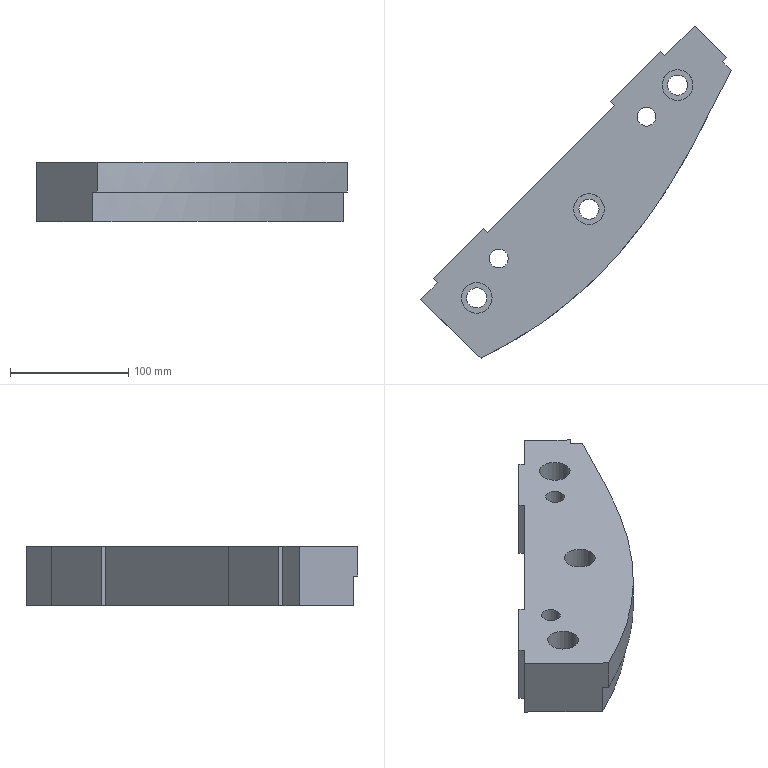Part | NX | features solid 2 | 1 solid | 32 faces | box 263.082 x 280.883 x 50 mm | volume 1203594 mm3 | plane 21 | cylinder 8 | spline 3 | commonest cylinder face diameters 17 x3 26 x3 16 x2
STEP:
#1=CARTESIAN_POINT('',(531.946,-303.622,-50.));
#2=VERTEX_POINT('',#1);
#3=CARTESIAN_POINT('',(528.349,-300.149,-50.));
#4=VERTEX_POINT('',#3);
#5=CARTESIAN_POINT('',(535.7,-307.247,-50.));
#6=DIRECTION('',(-0.7193,0.6947,0.));
#7=VECTOR('',#6,1000.);
#8=LINE('',#5,#7);
#9=EDGE_CURVE('',#2,#4,#8,.T.);
#10=ORIENTED_EDGE('',*,*,#9,.T.);
#11=CARTESIAN_POINT('',(528.349,-300.149,0.));
#12=VERTEX_POINT('',#11);
#13=CARTESIAN_POINT('',(528.349,-300.149,-50.));
#14=DIRECTION('',(0.,0.,1.));
#15=VECTOR('',#14,1000.);
#16=LINE('',#13,#15);
#17=EDGE_CURVE('',#4,#12,#16,.T.);
#18=ORIENTED_EDGE('',*,*,#17,.T.);
#19=CARTESIAN_POINT('',(535.7,-307.247,0.));
#20=VERTEX_POINT('',#19);
#21=CARTESIAN_POINT('',(535.7,-307.247,0.));
#22=DIRECTION('',(-0.7193,0.6947,0.));
#23=VECTOR('',#22,1000.);
#24=LINE('',#21,#23);
#25=EDGE_CURVE('',#20,#12,#24,.T.);
#26=ORIENTED_EDGE('',*,*,#25,.F.);
#27=CARTESIAN_POINT('',(535.7,-307.247,-25.));
#28=VERTEX_POINT('',#27);
#29=CARTESIAN_POINT('',(535.7,-307.247,-50.));
#30=DIRECTION('',(0.,0.,1.));
#31=VECTOR('',#30,1000.);
#32=LINE('',#29,#31);
#33=EDGE_CURVE('',#28,#20,#32,.T.);
#34=ORIENTED_EDGE('',*,*,#33,.F.);
#35=CARTESIAN_POINT('',(531.946,-303.622,-25.));
#36=VERTEX_POINT('',#35);
#37=CARTESIAN_POINT('',(535.7,-307.247,-25.));
#38=DIRECTION('',(0.7193,-0.6947,0.));
#39=VECTOR('',#38,1000.);
#40=LINE('',#37,#39);
#41=EDGE_CURVE('',#36,#28,#40,.T.);
#42=ORIENTED_EDGE('',*,*,#41,.F.);
#43=CARTESIAN_POINT('',(531.946,-303.622,-42.5));
#44=DIRECTION('',(0.,0.,-1.));
#45=VECTOR('',#44,1000.);
#46=LINE('',#43,#45);
#47=EDGE_CURVE('',#36,#2,#46,.T.);
#48=ORIENTED_EDGE('',*,*,#47,.T.);
#49=EDGE_LOOP('',(#10,#18,#26,#34,#42,#48));
#50=FACE_BOUND('',#49,.T.);
#51=CARTESIAN_POINT('',(535.7,-307.247,-50.));
#52=DIRECTION('',(0.6947,0.7193,0.));
#53=DIRECTION('',(-0.7193,0.6947,0.));
#54=AXIS2_PLACEMENT_3D('',#51,#52,#53);
#55=PLANE('',#54);
#56=ADVANCED_FACE('',(#50),#55,.T.);
#57=CARTESIAN_POINT('',(504.099,-269.78,-50.));
#58=VERTEX_POINT('',#57);
#59=CARTESIAN_POINT('',(479.349,-294.529,-50.));
#60=VERTEX_POINT('',#59);
#61=CARTESIAN_POINT('',(500.563,-273.316,-50.));
#62=DIRECTION('',(-0.7071,-0.7071,0.));
#63=VECTOR('',#62,1000.);
#64=LINE('',#61,#63);
#65=EDGE_CURVE('',#58,#60,#64,.T.);
#66=ORIENTED_EDGE('',*,*,#65,.T.);
#67=CARTESIAN_POINT('',(479.349,-294.529,0.));
#68=VERTEX_POINT('',#67);
#69=CARTESIAN_POINT('',(479.349,-294.529,-50.));
#70=DIRECTION('',(0.,0.,1.));
#71=VECTOR('',#70,1000.);
#72=LINE('',#69,#71);
#73=EDGE_CURVE('',#60,#68,#72,.T.);
#74=ORIENTED_EDGE('',*,*,#73,.T.);
#75=CARTESIAN_POINT('',(504.099,-269.78,0.));
#76=VERTEX_POINT('',#75);
#77=CARTESIAN_POINT('',(500.563,-273.316,0.));
#78=DIRECTION('',(-0.7071,-0.7071,0.));
#79=VECTOR('',#78,1000.);
#80=LINE('',#77,#79);
#81=EDGE_CURVE('',#76,#68,#80,.T.);
#82=ORIENTED_EDGE('',*,*,#81,.F.);
#83=CARTESIAN_POINT('',(504.099,-269.78,-50.));
#84=DIRECTION('',(0.,0.,1.));
#85=VECTOR('',#84,1000.);
#86=LINE('',#83,#85);
#87=EDGE_CURVE('',#58,#76,#86,.T.);
#88=ORIENTED_EDGE('',*,*,#87,.F.);
#89=EDGE_LOOP('',(#66,#74,#82,#88));
#90=FACE_BOUND('',#89,.T.);
#91=CARTESIAN_POINT('',(500.563,-273.316,-50.));
#92=DIRECTION('',(-0.7071,0.7071,0.));
#93=DIRECTION('',(-0.7071,-0.7071,0.));
#94=AXIS2_PLACEMENT_3D('',#91,#92,#93);
#95=PLANE('',#94);
#96=ADVANCED_FACE('',(#90),#95,.T.);
#97=CARTESIAN_POINT('',(436.923,-336.955,-50.));
#98=VERTEX_POINT('',#97);
#99=CARTESIAN_POINT('',(436.923,-336.955,0.));
#100=VERTEX_POINT('',#99);
#101=CARTESIAN_POINT('',(436.923,-336.955,-50.));
#102=DIRECTION('',(0.,0.,1.));
#103=VECTOR('',#102,1000.);
#104=LINE('',#101,#103);
#105=EDGE_CURVE('',#98,#100,#104,.T.);
#106=ORIENTED_EDGE('',*,*,#105,.F.);
#107=CARTESIAN_POINT('',(329.186,-444.692,-50.));
#108=VERTEX_POINT('',#107);
#109=CARTESIAN_POINT('',(500.563,-273.316,-50.));
#110=DIRECTION('',(-0.7071,-0.7071,0.));
#111=VECTOR('',#110,1000.);
#112=LINE('',#109,#111);
#113=EDGE_CURVE('',#98,#108,#112,.T.);
#114=ORIENTED_EDGE('',*,*,#113,.T.);
#115=CARTESIAN_POINT('',(329.186,-444.692,0.));
#116=VERTEX_POINT('',#115);
#117=CARTESIAN_POINT('',(329.186,-444.692,-50.));
#118=DIRECTION('',(0.,0.,1.));
#119=VECTOR('',#118,1000.);
#120=LINE('',#117,#119);
#121=EDGE_CURVE('',#108,#116,#120,.T.);
#122=ORIENTED_EDGE('',*,*,#121,.T.);
#123=CARTESIAN_POINT('',(500.563,-273.316,0.));
#124=DIRECTION('',(-0.7071,-0.7071,0.));
#125=VECTOR('',#124,1000.);
#126=LINE('',#123,#125);
#127=EDGE_CURVE('',#100,#116,#126,.T.);
#128=ORIENTED_EDGE('',*,*,#127,.F.);
#129=EDGE_LOOP('',(#106,#114,#122,#128));
#130=FACE_BOUND('',#129,.T.);
#131=CARTESIAN_POINT('',(500.563,-273.316,-50.));
#132=DIRECTION('',(-0.7071,0.7071,0.));
#133=DIRECTION('',(-0.7071,-0.7071,0.));
#134=AXIS2_PLACEMENT_3D('',#131,#132,#133);
#135=PLANE('',#134);
#136=ADVANCED_FACE('',(#130),#135,.T.);
#137=CARTESIAN_POINT('',(323.774,-550.663,-25.));
#138=VERTEX_POINT('',#137);
#139=CARTESIAN_POINT('',(319.947,-546.966,-25.));
#140=VERTEX_POINT('',#139);
#141=CARTESIAN_POINT('',(272.617,-501.261,-25.));
#142=DIRECTION('',(-0.7193,0.6947,0.));
#143=VECTOR('',#142,1000.);
#144=LINE('',#141,#143);
#145=EDGE_CURVE('',#138,#140,#144,.T.);
#146=ORIENTED_EDGE('',*,*,#145,.F.);
#147=CARTESIAN_POINT('',(323.774,-550.663,0.));
#148=VERTEX_POINT('',#147);
#149=CARTESIAN_POINT('',(323.774,-550.663,-50.));
#150=DIRECTION('',(0.,0.,1.));
#151=VECTOR('',#150,1000.);
#152=LINE('',#149,#151);
#153=EDGE_CURVE('',#138,#148,#152,.T.);
#154=ORIENTED_EDGE('',*,*,#153,.T.);
#155=CARTESIAN_POINT('',(272.617,-501.261,0.));
#156=VERTEX_POINT('',#155);
#157=CARTESIAN_POINT('',(272.617,-501.261,0.));
#158=DIRECTION('',(0.7193,-0.6947,0.));
#159=VECTOR('',#158,1000.);
#160=LINE('',#157,#159);
#161=EDGE_CURVE('',#156,#148,#160,.T.);
#162=ORIENTED_EDGE('',*,*,#161,.F.);
#163=CARTESIAN_POINT('',(272.617,-501.261,-50.));
#164=VERTEX_POINT('',#163);
#165=CARTESIAN_POINT('',(272.617,-501.261,-50.));
#166=DIRECTION('',(0.,0.,1.));
#167=VECTOR('',#166,1000.);
#168=LINE('',#165,#167);
#169=EDGE_CURVE('',#164,#156,#168,.T.);
#170=ORIENTED_EDGE('',*,*,#169,.F.);
#171=CARTESIAN_POINT('',(319.947,-546.966,-50.));
#172=VERTEX_POINT('',#171);
#173=CARTESIAN_POINT('',(272.617,-501.261,-50.));
#174=DIRECTION('',(0.7193,-0.6947,0.));
#175=VECTOR('',#174,1000.);
#176=LINE('',#173,#175);
#177=EDGE_CURVE('',#164,#172,#176,.T.);
#178=ORIENTED_EDGE('',*,*,#177,.T.);
#179=CARTESIAN_POINT('',(319.947,-546.966,-42.5));
#180=DIRECTION('',(0.,0.,-1.));
#181=VECTOR('',#180,1000.);
#182=LINE('',#179,#181);
#183=EDGE_CURVE('',#172,#140,#182,.F.);
#184=ORIENTED_EDGE('',*,*,#183,.T.);
#185=EDGE_LOOP('',(#146,#154,#162,#170,#178,#184));
#186=FACE_BOUND('',#185,.T.);
#187=CARTESIAN_POINT('',(272.617,-501.261,-50.));
#188=DIRECTION('',(-0.6947,-0.7193,0.));
#189=DIRECTION('',(0.7193,-0.6947,0.));
#190=AXIS2_PLACEMENT_3D('',#187,#188,#189);
#191=PLANE('',#190);
#192=ADVANCED_FACE('',(#186),#191,.T.);
#193=CARTESIAN_POINT('',(286.76,-487.119,-50.));
#194=VERTEX_POINT('',#193);
#195=CARTESIAN_POINT('',(286.76,-487.119,0.));
#196=VERTEX_POINT('',#195);
#197=CARTESIAN_POINT('',(286.76,-487.119,-50.));
#198=DIRECTION('',(0.,0.,1.));
#199=VECTOR('',#198,1000.);
#200=LINE('',#197,#199);
#201=EDGE_CURVE('',#194,#196,#200,.T.);
#202=ORIENTED_EDGE('',*,*,#201,.F.);
#203=CARTESIAN_POINT('',(500.563,-273.316,-50.));
#204=DIRECTION('',(-0.7071,-0.7071,0.));
#205=VECTOR('',#204,1000.);
#206=LINE('',#203,#205);
#207=EDGE_CURVE('',#194,#164,#206,.T.);
#208=ORIENTED_EDGE('',*,*,#207,.T.);
#209=ORIENTED_EDGE('',*,*,#169,.T.);
#210=CARTESIAN_POINT('',(500.563,-273.316,0.));
#211=DIRECTION('',(-0.7071,-0.7071,0.));
#212=VECTOR('',#211,1000.);
#213=LINE('',#210,#212);
#214=EDGE_CURVE('',#196,#156,#213,.T.);
#215=ORIENTED_EDGE('',*,*,#214,.F.);
#216=EDGE_LOOP('',(#202,#208,#209,#215));
#217=FACE_BOUND('',#216,.T.);
#218=CARTESIAN_POINT('',(500.563,-273.316,-50.));
#219=DIRECTION('',(-0.7071,0.7071,0.));
#220=DIRECTION('',(-0.7071,-0.7071,0.));
#221=AXIS2_PLACEMENT_3D('',#218,#219,#220);
#222=PLANE('',#221);
#223=ADVANCED_FACE('',(#217),#222,.T.);
#224=CARTESIAN_POINT('',(325.65,-441.157,-50.));
#225=VERTEX_POINT('',#224);
#226=CARTESIAN_POINT('',(325.65,-441.157,0.));
#227=VERTEX_POINT('',#226);
#228=CARTESIAN_POINT('',(325.65,-441.157,-50.));
#229=DIRECTION('',(0.,0.,1.));
#230=VECTOR('',#229,1000.);
#231=LINE('',#228,#230);
#232=EDGE_CURVE('',#225,#227,#231,.T.);
#233=ORIENTED_EDGE('',*,*,#232,.T.);
#234=CARTESIAN_POINT('',(329.186,-444.692,0.));
#235=DIRECTION('',(-0.7071,0.7071,0.));
#236=VECTOR('',#235,1000.);
#237=LINE('',#234,#236);
#238=EDGE_CURVE('',#116,#227,#237,.T.);
#239=ORIENTED_EDGE('',*,*,#238,.F.);
#240=ORIENTED_EDGE('',*,*,#121,.F.);
#241=CARTESIAN_POINT('',(329.186,-444.692,-50.));
#242=DIRECTION('',(-0.7071,0.7071,0.));
#243=VECTOR('',#242,1000.);
#244=LINE('',#241,#243);
#245=EDGE_CURVE('',#108,#225,#244,.T.);
#246=ORIENTED_EDGE('',*,*,#245,.T.);
#247=EDGE_LOOP('',(#233,#239,#240,#246));
#248=FACE_BOUND('',#247,.T.);
#249=CARTESIAN_POINT('',(329.186,-444.692,-50.));
#250=DIRECTION('',(-0.7071,-0.7071,0.));
#251=DIRECTION('',(0.7071,-0.7071,0.));
#252=AXIS2_PLACEMENT_3D('',#249,#250,#251);
#253=PLANE('',#252);
#254=ADVANCED_FACE('',(#248),#253,.F.);
#255=CARTESIAN_POINT('',(283.224,-483.583,-50.));
#256=VERTEX_POINT('',#255);
#257=CARTESIAN_POINT('',(283.224,-483.583,0.));
#258=VERTEX_POINT('',#257);
#259=CARTESIAN_POINT('',(283.224,-483.583,-50.));
#260=DIRECTION('',(0.,0.,1.));
#261=VECTOR('',#260,1000.);
#262=LINE('',#259,#261);
#263=EDGE_CURVE('',#256,#258,#262,.T.);
#264=ORIENTED_EDGE('',*,*,#263,.F.);
#265=CARTESIAN_POINT('',(286.76,-487.119,-50.));
#266=DIRECTION('',(-0.7071,0.7071,0.));
#267=VECTOR('',#266,1000.);
#268=LINE('',#265,#267);
#269=EDGE_CURVE('',#194,#256,#268,.T.);
#270=ORIENTED_EDGE('',*,*,#269,.F.);
#271=ORIENTED_EDGE('',*,*,#201,.T.);
#272=CARTESIAN_POINT('',(286.76,-487.119,0.));
#273=DIRECTION('',(-0.7071,0.7071,0.));
#274=VECTOR('',#273,1000.);
#275=LINE('',#272,#274);
#276=EDGE_CURVE('',#196,#258,#275,.T.);
#277=ORIENTED_EDGE('',*,*,#276,.T.);
#278=EDGE_LOOP('',(#264,#270,#271,#277));
#279=FACE_BOUND('',#278,.T.);
#280=CARTESIAN_POINT('',(286.76,-487.119,-50.));
#281=DIRECTION('',(-0.7071,-0.7071,0.));
#282=DIRECTION('',(0.7071,-0.7071,0.));
#283=AXIS2_PLACEMENT_3D('',#280,#281,#282);
#284=PLANE('',#283);
#285=ADVANCED_FACE('',(#279),#284,.T.);
#286=CARTESIAN_POINT('',(325.65,-441.157,0.));
#287=DIRECTION('',(-0.7071,-0.7071,0.));
#288=VECTOR('',#287,1000.);
#289=LINE('',#286,#288);
#290=EDGE_CURVE('',#227,#258,#289,.T.);
#291=ORIENTED_EDGE('',*,*,#290,.F.);
#292=ORIENTED_EDGE('',*,*,#232,.F.);
#293=CARTESIAN_POINT('',(325.65,-441.157,-50.));
#294=DIRECTION('',(-0.7071,-0.7071,0.));
#295=VECTOR('',#294,1000.);
#296=LINE('',#293,#295);
#297=EDGE_CURVE('',#225,#256,#296,.T.);
#298=ORIENTED_EDGE('',*,*,#297,.T.);
#299=ORIENTED_EDGE('',*,*,#263,.T.);
#300=EDGE_LOOP('',(#291,#292,#298,#299));
#301=FACE_BOUND('',#300,.T.);
#302=CARTESIAN_POINT('',(325.65,-441.157,-50.));
#303=DIRECTION('',(-0.7071,0.7071,0.));
#304=DIRECTION('',(-0.7071,-0.7071,0.));
#305=AXIS2_PLACEMENT_3D('',#302,#303,#304);
#306=PLANE('',#305);
#307=ADVANCED_FACE('',(#301),#306,.T.);
#308=CARTESIAN_POINT('',(475.814,-290.993,-50.));
#309=VERTEX_POINT('',#308);
#310=CARTESIAN_POINT('',(475.814,-290.993,0.));
#311=VERTEX_POINT('',#310);
#312=CARTESIAN_POINT('',(475.814,-290.993,-50.));
#313=DIRECTION('',(0.,0.,1.));
#314=VECTOR('',#313,1000.);
#315=LINE('',#312,#314);
#316=EDGE_CURVE('',#309,#311,#315,.T.);
#317=ORIENTED_EDGE('',*,*,#316,.T.);
#318=CARTESIAN_POINT('',(479.349,-294.529,0.));
#319=DIRECTION('',(-0.7071,0.7071,0.));
#320=VECTOR('',#319,1000.);
#321=LINE('',#318,#320);
#322=EDGE_CURVE('',#68,#311,#321,.T.);
#323=ORIENTED_EDGE('',*,*,#322,.F.);
#324=ORIENTED_EDGE('',*,*,#73,.F.);
#325=CARTESIAN_POINT('',(479.349,-294.529,-50.));
#326=DIRECTION('',(-0.7071,0.7071,0.));
#327=VECTOR('',#326,1000.);
#328=LINE('',#325,#327);
#329=EDGE_CURVE('',#60,#309,#328,.T.);
#330=ORIENTED_EDGE('',*,*,#329,.T.);
#331=EDGE_LOOP('',(#317,#323,#324,#330));
#332=FACE_BOUND('',#331,.T.);
#333=CARTESIAN_POINT('',(479.349,-294.529,-50.));
#334=DIRECTION('',(-0.7071,-0.7071,0.));
#335=DIRECTION('',(0.7071,-0.7071,0.));
#336=AXIS2_PLACEMENT_3D('',#333,#334,#335);
#337=PLANE('',#336);
#338=ADVANCED_FACE('',(#332),#337,.F.);
#339=CARTESIAN_POINT('',(433.388,-333.42,-50.));
#340=VERTEX_POINT('',#339);
#341=CARTESIAN_POINT('',(433.388,-333.42,0.));
#342=VERTEX_POINT('',#341);
#343=CARTESIAN_POINT('',(433.388,-333.42,-50.));
#344=DIRECTION('',(0.,0.,1.));
#345=VECTOR('',#344,1000.);
#346=LINE('',#343,#345);
#347=EDGE_CURVE('',#340,#342,#346,.T.);
#348=ORIENTED_EDGE('',*,*,#347,.F.);
#349=CARTESIAN_POINT('',(436.923,-336.955,-50.));
#350=DIRECTION('',(-0.7071,0.7071,0.));
#351=VECTOR('',#350,1000.);
#352=LINE('',#349,#351);
#353=EDGE_CURVE('',#98,#340,#352,.T.);
#354=ORIENTED_EDGE('',*,*,#353,.F.);
#355=ORIENTED_EDGE('',*,*,#105,.T.);
#356=CARTESIAN_POINT('',(436.923,-336.955,0.));
#357=DIRECTION('',(-0.7071,0.7071,0.));
#358=VECTOR('',#357,1000.);
#359=LINE('',#356,#358);
#360=EDGE_CURVE('',#100,#342,#359,.T.);
#361=ORIENTED_EDGE('',*,*,#360,.T.);
#362=EDGE_LOOP('',(#348,#354,#355,#361));
#363=FACE_BOUND('',#362,.T.);
#364=CARTESIAN_POINT('',(436.923,-336.955,-50.));
#365=DIRECTION('',(-0.7071,-0.7071,0.));
#366=DIRECTION('',(0.7071,-0.7071,0.));
#367=AXIS2_PLACEMENT_3D('',#364,#365,#366);
#368=PLANE('',#367);
#369=ADVANCED_FACE('',(#363),#368,.T.);
#370=CARTESIAN_POINT('',(497.027,-269.78,0.));
#371=DIRECTION('',(-0.7071,-0.7071,0.));
#372=VECTOR('',#371,1000.);
#373=LINE('',#370,#372);
#374=EDGE_CURVE('',#311,#342,#373,.T.);
#375=ORIENTED_EDGE('',*,*,#374,.F.);
#376=ORIENTED_EDGE('',*,*,#316,.F.);
#377=CARTESIAN_POINT('',(497.027,-269.78,-50.));
#378=DIRECTION('',(-0.7071,-0.7071,0.));
#379=VECTOR('',#378,1000.);
#380=LINE('',#377,#379);
#381=EDGE_CURVE('',#309,#340,#380,.T.);
#382=ORIENTED_EDGE('',*,*,#381,.T.);
#383=ORIENTED_EDGE('',*,*,#347,.T.);
#384=EDGE_LOOP('',(#375,#376,#382,#383));
#385=FACE_BOUND('',#384,.T.);
#386=CARTESIAN_POINT('',(497.027,-269.78,-50.));
#387=DIRECTION('',(-0.7071,0.7071,0.));
#388=DIRECTION('',(-0.7071,-0.7071,0.));
#389=AXIS2_PLACEMENT_3D('',#386,#387,#388);
#390=PLANE('',#389);
#391=ADVANCED_FACE('',(#385),#390,.T.);
#392=CARTESIAN_POINT('',(471.782,-346.506,0.));
#393=VERTEX_POINT('',#392);
#394=CARTESIAN_POINT('',(463.782,-346.506,0.));
#395=DIRECTION('',(0.,0.,1.));
#396=DIRECTION('',(1.,0.,0.));
#397=AXIS2_PLACEMENT_3D('',#394,#395,#396);
#398=CIRCLE('',#397,8.);
#399=EDGE_CURVE('',#393,#393,#398,.T.);
#400=ORIENTED_EDGE('',*,*,#399,.F.);
#401=EDGE_LOOP('',(#400));
#402=FACE_BOUND('',#401,.T.);
#403=CARTESIAN_POINT('',(346.782,-466.506,0.));
#404=VERTEX_POINT('',#403);
#405=CARTESIAN_POINT('',(338.782,-466.506,0.));
#406=DIRECTION('',(0.,0.,1.));
#407=DIRECTION('',(1.,0.,0.));
#408=AXIS2_PLACEMENT_3D('',#405,#406,#407);
#409=CIRCLE('',#408,8.);
#410=EDGE_CURVE('',#404,#404,#409,.T.);
#411=ORIENTED_EDGE('',*,*,#410,.F.);
#412=EDGE_LOOP('',(#411));
#413=FACE_BOUND('',#412,.T.);
#414=ORIENTED_EDGE('',*,*,#161,.T.);
#415=CARTESIAN_POINT('',(535.7,-307.247,0.));
#416=CARTESIAN_POINT('',(534.934,-308.728,0.));
#417=CARTESIAN_POINT('',(529.574,-319.09,0.));
#418=CARTESIAN_POINT('',(521.917,-333.894,0.));
#419=CARTESIAN_POINT('',(512.728,-351.658,0.));
#420=CARTESIAN_POINT('',(506.903,-362.951,0.));
#421=CARTESIAN_POINT('',(499.555,-376.977,0.));
#422=CARTESIAN_POINT('',(488.977,-395.893,0.));
#423=CARTESIAN_POINT('',(467.289,-430.253,0.));
#424=CARTESIAN_POINT('',(433.523,-472.816,0.));
#425=CARTESIAN_POINT('',(392.995,-509.066,0.));
#426=CARTESIAN_POINT('',(357.027,-533.308,0.));
#427=CARTESIAN_POINT('',(337.263,-544.104,0.));
#428=CARTESIAN_POINT('',(326.021,-549.566,0.));
#429=CARTESIAN_POINT('',(324.523,-550.297,0.));
#430=CARTESIAN_POINT('',(323.774,-550.663,0.));
#431=B_SPLINE_CURVE_WITH_KNOTS('',3,(#415,#416,#417,#418,#419,#420,#421,#422,#423,#424,#425,#426,#427,#428,#429,#430),.UNSPECIFIED.,.F.,.F.,(4,1,1,1,1,1,1,1,1,1,1,1,1,4),(0.,0.01516,0.1061,0.1516,0.197,0.2216,0.2955,0.394,0.5909,0.7879,0.8864,0.9848,0.9924,1.),.UNSPECIFIED.);
#432=EDGE_CURVE('',#20,#148,#431,.T.);
#433=ORIENTED_EDGE('',*,*,#432,.F.);
#434=ORIENTED_EDGE('',*,*,#25,.T.);
#435=CARTESIAN_POINT('',(531.822,-296.552,0.));
#436=VERTEX_POINT('',#435);
#437=CARTESIAN_POINT('',(531.822,-296.552,0.));
#438=DIRECTION('',(-0.6947,-0.7193,0.));
#439=VECTOR('',#438,1000.);
#440=LINE('',#437,#439);
#441=EDGE_CURVE('',#436,#12,#440,.T.);
#442=ORIENTED_EDGE('',*,*,#441,.F.);
#443=CARTESIAN_POINT('',(539.173,-303.651,0.));
#444=DIRECTION('',(-0.7193,0.6947,0.));
#445=VECTOR('',#444,1000.);
#446=LINE('',#443,#445);
#447=EDGE_CURVE('',#436,#76,#446,.T.);
#448=ORIENTED_EDGE('',*,*,#447,.T.);
#449=ORIENTED_EDGE('',*,*,#81,.T.);
#450=ORIENTED_EDGE('',*,*,#322,.T.);
#451=ORIENTED_EDGE('',*,*,#374,.T.);
#452=ORIENTED_EDGE('',*,*,#360,.F.);
#453=ORIENTED_EDGE('',*,*,#127,.T.);
#454=ORIENTED_EDGE('',*,*,#238,.T.);
#455=ORIENTED_EDGE('',*,*,#290,.T.);
#456=ORIENTED_EDGE('',*,*,#276,.F.);
#457=ORIENTED_EDGE('',*,*,#214,.T.);
#458=EDGE_LOOP('',(#414,#433,#434,#442,#448,#449,#450,#451,#452,#453,#454,#455,#456,#457));
#459=FACE_BOUND('',#458,.T.);
#460=CARTESIAN_POINT('',(307.122,-499.794,0.));
#461=VERTEX_POINT('',#460);
#462=CARTESIAN_POINT('',(320.122,-499.794,0.));
#463=DIRECTION('',(0.,0.,-1.));
#464=DIRECTION('',(-1.,0.,0.));
#465=AXIS2_PLACEMENT_3D('',#462,#463,#464);
#466=CIRCLE('',#465,13.);
#467=EDGE_CURVE('',#461,#461,#466,.T.);
#468=ORIENTED_EDGE('',*,*,#467,.T.);
#469=EDGE_LOOP('',(#468));
#470=FACE_BOUND('',#469,.T.);
#471=CARTESIAN_POINT('',(477.122,-319.794,0.));
#472=VERTEX_POINT('',#471);
#473=CARTESIAN_POINT('',(490.122,-319.794,0.));
#474=DIRECTION('',(0.,0.,-1.));
#475=DIRECTION('',(-1.,0.,0.));
#476=AXIS2_PLACEMENT_3D('',#473,#474,#475);
#477=CIRCLE('',#476,13.);
#478=EDGE_CURVE('',#472,#472,#477,.T.);
#479=ORIENTED_EDGE('',*,*,#478,.T.);
#480=EDGE_LOOP('',(#479));
#481=FACE_BOUND('',#480,.T.);
#482=CARTESIAN_POINT('',(402.122,-424.794,0.));
#483=VERTEX_POINT('',#482);
#484=CARTESIAN_POINT('',(415.122,-424.794,0.));
#485=DIRECTION('',(0.,0.,-1.));
#486=DIRECTION('',(-1.,0.,0.));
#487=AXIS2_PLACEMENT_3D('',#484,#485,#486);
#488=CIRCLE('',#487,13.);
#489=EDGE_CURVE('',#483,#483,#488,.T.);
#490=ORIENTED_EDGE('',*,*,#489,.T.);
#491=EDGE_LOOP('',(#490));
#492=FACE_BOUND('',#491,.T.);
#493=CARTESIAN_POINT('',(484.874,-308.369,0.));
#494=DIRECTION('',(0.,0.,1.));
#495=DIRECTION('',(1.,0.,0.));
#496=AXIS2_PLACEMENT_3D('',#493,#494,#495);
#497=PLANE('',#496);
#498=ADVANCED_FACE('',(#402,#413,#459,#470,#481,#492),#497,.T.);
#499=CARTESIAN_POINT('',(471.782,-346.506,-50.));
#500=VERTEX_POINT('',#499);
#501=CARTESIAN_POINT('',(463.782,-346.506,-50.));
#502=DIRECTION('',(0.,0.,1.));
#503=DIRECTION('',(1.,0.,0.));
#504=AXIS2_PLACEMENT_3D('',#501,#502,#503);
#505=CIRCLE('',#504,8.);
#506=EDGE_CURVE('',#500,#500,#505,.T.);
#507=ORIENTED_EDGE('',*,*,#506,.T.);
#508=EDGE_LOOP('',(#507));
#509=FACE_BOUND('',#508,.T.);
#510=CARTESIAN_POINT('',(346.782,-466.506,-50.));
#511=VERTEX_POINT('',#510);
#512=CARTESIAN_POINT('',(338.782,-466.506,-50.));
#513=DIRECTION('',(0.,0.,1.));
#514=DIRECTION('',(1.,0.,0.));
#515=AXIS2_PLACEMENT_3D('',#512,#513,#514);
#516=CIRCLE('',#515,8.);
#517=EDGE_CURVE('',#511,#511,#516,.T.);
#518=ORIENTED_EDGE('',*,*,#517,.T.);
#519=EDGE_LOOP('',(#518));
#520=FACE_BOUND('',#519,.T.);
#521=CARTESIAN_POINT('',(481.622,-319.794,-50.));
#522=VERTEX_POINT('',#521);
#523=CARTESIAN_POINT('',(490.122,-319.794,-50.));
#524=DIRECTION('',(0.,0.,-1.));
#525=DIRECTION('',(-1.,0.,0.));
#526=AXIS2_PLACEMENT_3D('',#523,#524,#525);
#527=CIRCLE('',#526,8.5);
#528=EDGE_CURVE('',#522,#522,#527,.T.);
#529=ORIENTED_EDGE('',*,*,#528,.F.);
#530=EDGE_LOOP('',(#529));
#531=FACE_BOUND('',#530,.T.);
#532=CARTESIAN_POINT('',(531.946,-303.622,-50.));
#533=CARTESIAN_POINT('',(528.899,-309.512,-50.));
#534=CARTESIAN_POINT('',(524.876,-317.289,-50.));
#535=CARTESIAN_POINT('',(520.608,-325.541,-50.));
#536=CARTESIAN_POINT('',(517.954,-330.671,-50.));
#537=CARTESIAN_POINT('',(516.199,-334.064,-50.));
#538=CARTESIAN_POINT('',(515.069,-336.249,-50.));
#539=CARTESIAN_POINT('',(514.358,-337.623,-50.));
#540=CARTESIAN_POINT('',(513.784,-338.732,-50.));
#541=CARTESIAN_POINT('',(513.42,-339.436,-50.));
#542=CARTESIAN_POINT('',(513.197,-339.867,-50.));
#543=CARTESIAN_POINT('',(513.087,-340.081,-50.));
#544=CARTESIAN_POINT('',(513.015,-340.22,-50.));
#545=CARTESIAN_POINT('',(512.971,-340.305,-50.));
#546=CARTESIAN_POINT('',(512.938,-340.37,-50.));
#547=CARTESIAN_POINT('',(512.925,-340.394,-50.));
#548=CARTESIAN_POINT('',(512.908,-340.427,-50.));
#549=CARTESIAN_POINT('',(512.927,-340.39,-50.));
#550=CARTESIAN_POINT('',(512.828,-340.582,-50.));
#551=CARTESIAN_POINT('',(512.737,-340.758,-50.));
#552=CARTESIAN_POINT('',(512.558,-341.104,-50.));
#553=CARTESIAN_POINT('',(512.313,-341.577,-50.));
#554=CARTESIAN_POINT('',(512.015,-342.154,-50.));
#555=CARTESIAN_POINT('',(511.618,-342.92,-50.));
#556=CARTESIAN_POINT('',(511.123,-343.879,-50.));
#557=CARTESIAN_POINT('',(510.33,-345.413,-50.));
#558=CARTESIAN_POINT('',(509.338,-347.33,-50.));
#559=CARTESIAN_POINT('',(507.753,-350.397,-50.));
#560=CARTESIAN_POINT('',(506.164,-353.471,-50.));
#561=CARTESIAN_POINT('',(504.784,-356.142,-50.));
#562=CARTESIAN_POINT('',(503.98,-357.698,-50.));
#563=CARTESIAN_POINT('',(503.42,-358.781,-50.));
#564=CARTESIAN_POINT('',(502.695,-360.183,-50.));
#565=CARTESIAN_POINT('',(501.804,-361.9,-50.));
#566=CARTESIAN_POINT('',(500.253,-364.873,-50.));
#567=CARTESIAN_POINT('',(498.163,-368.84,-50.));
#568=CARTESIAN_POINT('',(496.204,-372.499,-50.));
#569=CARTESIAN_POINT('',(494.922,-374.861,-50.));
#570=CARTESIAN_POINT('',(494.191,-376.198,-50.));
#571=CARTESIAN_POINT('',(493.71,-377.073,-50.));
#572=CARTESIAN_POINT('',(493.022,-378.318,-50.));
#573=CARTESIAN_POINT('',(492.175,-379.841,-50.));
#574=CARTESIAN_POINT('',(490.655,-382.554,-50.));
#575=CARTESIAN_POINT('',(488.487,-386.357,-50.));
#576=CARTESIAN_POINT('',(485.858,-390.869,-50.));
#577=CARTESIAN_POINT('',(482.326,-396.795,-50.));
#578=CARTESIAN_POINT('',(478.759,-402.579,-50.));
#579=CARTESIAN_POINT('',(475.128,-408.266,-50.));
#580=CARTESIAN_POINT('',(472.446,-412.374,-50.));
#581=CARTESIAN_POINT('',(469.506,-416.77,-50.));
#582=CARTESIAN_POINT('',(465.619,-422.435,-50.));
#583=CARTESIAN_POINT('',(460.645,-429.421,-50.));
#584=CARTESIAN_POINT('',(455.579,-436.191,-50.));
#585=CARTESIAN_POINT('',(451.43,-441.53,-50.));
#586=CARTESIAN_POINT('',(448.356,-445.39,-50.));
#587=CARTESIAN_POINT('',(444.971,-449.533,-50.));
#588=CARTESIAN_POINT('',(440.497,-454.858,-50.));
#589=CARTESIAN_POINT('',(432.482,-464.025,-50.));
#590=CARTESIAN_POINT('',(420.65,-476.497,-50.));
#591=CARTESIAN_POINT('',(408.263,-488.193,-50.));
#592=CARTESIAN_POINT('',(399.322,-495.954,-50.));
#593=CARTESIAN_POINT('',(394.113,-500.284,-50.));
#594=CARTESIAN_POINT('',(390.217,-503.432,-50.));
#595=CARTESIAN_POINT('',(386.083,-506.675,-50.));
#596=CARTESIAN_POINT('',(380.59,-510.854,-50.));
#597=CARTESIAN_POINT('',(373.601,-515.932,-50.));
#598=CARTESIAN_POINT('',(365.07,-521.751,-50.));
#599=CARTESIAN_POINT('',(356.378,-527.309,-50.));
#600=CARTESIAN_POINT('',(349.015,-531.712,-50.));
#601=CARTESIAN_POINT('',(343.02,-535.119,-50.));
#602=CARTESIAN_POINT('',(339.218,-537.205,-50.));
#603=CARTESIAN_POINT('',(336.183,-538.828,-50.));
#604=CARTESIAN_POINT('',(334.272,-539.832,-50.));
#605=CARTESIAN_POINT('',(332.74,-540.627,-50.));
#606=CARTESIAN_POINT('',(331.584,-541.22,-50.));
#607=CARTESIAN_POINT('',(330.628,-541.707,-50.));
#608=CARTESIAN_POINT('',(329.939,-542.056,-50.));
#609=CARTESIAN_POINT('',(329.573,-542.24,-50.));
#610=CARTESIAN_POINT('',(329.219,-542.418,-50.));
#611=CARTESIAN_POINT('',(329.17,-542.443,-50.));
#612=CARTESIAN_POINT('',(328.979,-542.539,-50.));
#613=CARTESIAN_POINT('',(328.656,-542.699,-50.));
#614=CARTESIAN_POINT('',(328.054,-542.997,-50.));
#615=CARTESIAN_POINT('',(327.163,-543.436,-50.));
#616=CARTESIAN_POINT('',(325.729,-544.141,-50.));
#617=CARTESIAN_POINT('',(323.485,-545.239,-50.));
#618=CARTESIAN_POINT('',(321.207,-546.352,-50.));
#619=CARTESIAN_POINT('',(319.947,-546.966,-50.));
#620=B_SPLINE_CURVE_WITH_KNOTS('',3,(#532,#533,#534,#535,#536,#537,#538,#539,#540,#541,#542,#543,#544,#545,#546,#547,#548,#549,#550,#551,#552,#553,#554,#555,#556,#557,#558,#559,#560,#561,#562,#563,#564,#565,#566,#567,#568,#569,#570,#571,#572,#573,#574,#575,#576,#577,#578,#579,#580,#581,#582,#583,#584,#585,#586,#587,#588,#589,#590,#591,#592,#593,#594,#595,#596,#597,#598,#599,#600,#601,#602,#603,#604,#605,#606,#607,#608,#609,#610,#611,#612,#613,#614,#615,#616,#617,#618,#619),.UNSPECIFIED.,.F.,.F.,(4,1,1,1,1,1,1,1,1,1,1,1,1,1,1,1,1,1,1,1,1,1,1,1,1,1,1,1,1,1,1,1,1,1,1,1,1,1,1,1,1,1,1,1,1,1,1,1,1,1,1,1,1,1,1,1,1,1,1,1,1,1,1,1,1,1,1,1,1,1,1,1,1,1,1,1,1,1,1,1,1,1,1,1,1,4),(0.,0.03125,0.04688,0.0625,0.07812,0.08594,0.09375,0.1016,0.1094,0.1133,0.1172,0.1191,0.1211,0.123,0.124,0.1245,0.125,0.1255,0.126,0.127,0.1289,0.1309,0.1328,0.1367,0.1406,0.1484,0.1562,0.1719,0.1797,0.1836,0.1875,0.1914,0.1953,0.2031,0.2188,0.2344,0.2422,0.2461,0.25,0.2539,0.2578,0.2656,0.2812,0.2969,0.3125,0.3438,0.3594,0.375,0.3906,0.4062,0.4375,0.4688,0.4844,0.5,0.5156,0.5312,0.5625,0.625,0.6875,0.7188,0.7344,0.75,0.7656,0.7812,0.8125,0.8438,0.875,0.9062,0.9219,0.9375,0.9453,0.9531,0.957,0.9609,0.9648,0.9668,0.9678,0.9688,0.9697,0.9707,0.9727,0.9766,0.9805,0.9844,0.9922,1.),.UNSPECIFIED.);
#621=EDGE_CURVE('',#2,#172,#620,.T.);
#622=ORIENTED_EDGE('',*,*,#621,.T.);
#623=ORIENTED_EDGE('',*,*,#177,.F.);
#624=ORIENTED_EDGE('',*,*,#207,.F.);
#625=ORIENTED_EDGE('',*,*,#269,.T.);
#626=ORIENTED_EDGE('',*,*,#297,.F.);
#627=ORIENTED_EDGE('',*,*,#245,.F.);
#628=ORIENTED_EDGE('',*,*,#113,.F.);
#629=ORIENTED_EDGE('',*,*,#353,.T.);
#630=ORIENTED_EDGE('',*,*,#381,.F.);
#631=ORIENTED_EDGE('',*,*,#329,.F.);
#632=ORIENTED_EDGE('',*,*,#65,.F.);
#633=CARTESIAN_POINT('',(531.822,-296.552,-50.));
#634=VERTEX_POINT('',#633);
#635=CARTESIAN_POINT('',(539.173,-303.651,-50.));
#636=DIRECTION('',(-0.7193,0.6947,0.));
#637=VECTOR('',#636,1000.);
#638=LINE('',#635,#637);
#639=EDGE_CURVE('',#634,#58,#638,.T.);
#640=ORIENTED_EDGE('',*,*,#639,.F.);
#641=CARTESIAN_POINT('',(531.822,-296.552,-50.));
#642=DIRECTION('',(-0.6947,-0.7193,0.));
#643=VECTOR('',#642,1000.);
#644=LINE('',#641,#643);
#645=EDGE_CURVE('',#634,#4,#644,.T.);
#646=ORIENTED_EDGE('',*,*,#645,.T.);
#647=ORIENTED_EDGE('',*,*,#9,.F.);
#648=EDGE_LOOP('',(#622,#623,#624,#625,#626,#627,#628,#629,#630,#631,#632,#640,#646,#647));
#649=FACE_BOUND('',#648,.T.);
#650=CARTESIAN_POINT('',(406.622,-424.794,-50.));
#651=VERTEX_POINT('',#650);
#652=CARTESIAN_POINT('',(415.122,-424.794,-50.));
#653=DIRECTION('',(0.,0.,-1.));
#654=DIRECTION('',(-1.,0.,0.));
#655=AXIS2_PLACEMENT_3D('',#652,#653,#654);
#656=CIRCLE('',#655,8.5);
#657=EDGE_CURVE('',#651,#651,#656,.T.);
#658=ORIENTED_EDGE('',*,*,#657,.F.);
#659=EDGE_LOOP('',(#658));
#660=FACE_BOUND('',#659,.T.);
#661=CARTESIAN_POINT('',(311.622,-499.794,-50.));
#662=VERTEX_POINT('',#661);
#663=CARTESIAN_POINT('',(320.122,-499.794,-50.));
#664=DIRECTION('',(0.,0.,-1.));
#665=DIRECTION('',(-1.,0.,0.));
#666=AXIS2_PLACEMENT_3D('',#663,#664,#665);
#667=CIRCLE('',#666,8.5);
#668=EDGE_CURVE('',#662,#662,#667,.T.);
#669=ORIENTED_EDGE('',*,*,#668,.F.);
#670=EDGE_LOOP('',(#669));
#671=FACE_BOUND('',#670,.T.);
#672=CARTESIAN_POINT('',(588.464,-1243.238,-50.));
#673=DIRECTION('',(0.,0.,1.));
#674=DIRECTION('',(1.,0.,0.));
#675=AXIS2_PLACEMENT_3D('',#672,#673,#674);
#676=PLANE('',#675);
#677=ADVANCED_FACE('',(#509,#520,#531,#649,#660,#671),#676,.F.);
#678=CARTESIAN_POINT('',(461.602,-428.037,-25.));
#679=VERTEX_POINT('',#678);
#680=CARTESIAN_POINT('',(382.529,-509.369,-25.));
#681=VERTEX_POINT('',#680);
#682=CARTESIAN_POINT('',(461.602,-428.037,-25.));
#683=CARTESIAN_POINT('',(450.453,-443.433,-25.));
#684=CARTESIAN_POINT('',(426.143,-472.723,-25.));
#685=CARTESIAN_POINT('',(397.676,-497.971,-25.));
#686=CARTESIAN_POINT('',(382.529,-509.369,-25.));
#687=B_SPLINE_CURVE_WITH_KNOTS('',3,(#682,#683,#684,#685,#686),.UNSPECIFIED.,.F.,.F.,(4,1,4),(0.4314,0.6062,0.781),.UNSPECIFIED.);
#688=EDGE_CURVE('',#679,#681,#687,.T.);
#689=ORIENTED_EDGE('',*,*,#688,.F.);
#690=CARTESIAN_POINT('',(481.498,-407.572,-25.));
#691=VERTEX_POINT('',#690);
#692=CARTESIAN_POINT('',(529.404,-358.298,-25.));
#693=DIRECTION('',(0.6971,0.717,0.));
#694=VECTOR('',#693,1000.);
#695=LINE('',#692,#694);
#696=EDGE_CURVE('',#679,#691,#695,.T.);
#697=ORIENTED_EDGE('',*,*,#696,.T.);
#698=CARTESIAN_POINT('',(465.438,-431.264,-25.));
#699=VERTEX_POINT('',#698);
#700=CARTESIAN_POINT('',(535.7,-307.247,-25.));
#701=CARTESIAN_POINT('',(534.934,-308.728,-25.));
#702=CARTESIAN_POINT('',(529.574,-319.09,-25.));
#703=CARTESIAN_POINT('',(521.917,-333.894,-25.));
#704=CARTESIAN_POINT('',(512.728,-351.658,-25.));
#705=CARTESIAN_POINT('',(506.903,-362.951,-25.));
#706=CARTESIAN_POINT('',(499.555,-376.977,-25.));
#707=CARTESIAN_POINT('',(488.977,-395.893,-25.));
#708=CARTESIAN_POINT('',(467.289,-430.253,-25.));
#709=CARTESIAN_POINT('',(433.523,-472.816,-25.));
#710=CARTESIAN_POINT('',(392.995,-509.066,-25.));
#711=CARTESIAN_POINT('',(357.027,-533.308,-25.));
#712=CARTESIAN_POINT('',(337.263,-544.104,-25.));
#713=CARTESIAN_POINT('',(326.021,-549.566,-25.));
#714=CARTESIAN_POINT('',(324.523,-550.297,-25.));
#715=CARTESIAN_POINT('',(323.774,-550.663,-25.));
#716=B_SPLINE_CURVE_WITH_KNOTS('',3,(#700,#701,#702,#703,#704,#705,#706,#707,#708,#709,#710,#711,#712,#713,#714,#715),.UNSPECIFIED.,.F.,.F.,(4,1,1,1,1,1,1,1,1,1,1,1,1,4),(0.,0.01516,0.1061,0.1516,0.197,0.2216,0.2955,0.394,0.5909,0.7879,0.8864,0.9848,0.9924,1.),.UNSPECIFIED.);
#717=EDGE_CURVE('',#699,#691,#716,.F.);
#718=ORIENTED_EDGE('',*,*,#717,.F.);
#719=CARTESIAN_POINT('',(385.845,-513.131,-25.));
#720=VERTEX_POINT('',#719);
#721=CARTESIAN_POINT('',(465.438,-431.264,-25.));
#722=CARTESIAN_POINT('',(438.907,-458.553,-25.));
#723=CARTESIAN_POINT('',(412.376,-485.842,-25.));
#724=CARTESIAN_POINT('',(385.845,-513.131,-25.));
#725=B_SPLINE_CURVE_WITH_KNOTS('',3,(#721,#722,#723,#724),.UNSPECIFIED.,.F.,.F.,(4,4),(0.5294,0.6436),.UNSPECIFIED.);
#726=EDGE_CURVE('',#699,#720,#725,.T.);
#727=ORIENTED_EDGE('',*,*,#726,.T.);
#728=CARTESIAN_POINT('',(364.19,-528.232,-25.));
#729=VERTEX_POINT('',#728);
#730=CARTESIAN_POINT('',(535.7,-307.247,-25.));
#731=CARTESIAN_POINT('',(534.934,-308.728,-25.));
#732=CARTESIAN_POINT('',(529.574,-319.09,-25.));
#733=CARTESIAN_POINT('',(521.917,-333.894,-25.));
#734=CARTESIAN_POINT('',(512.728,-351.658,-25.));
#735=CARTESIAN_POINT('',(506.903,-362.951,-25.));
#736=CARTESIAN_POINT('',(499.555,-376.977,-25.));
#737=CARTESIAN_POINT('',(488.977,-395.893,-25.));
#738=CARTESIAN_POINT('',(467.289,-430.253,-25.));
#739=CARTESIAN_POINT('',(433.523,-472.816,-25.));
#740=CARTESIAN_POINT('',(392.995,-509.066,-25.));
#741=CARTESIAN_POINT('',(357.027,-533.308,-25.));
#742=CARTESIAN_POINT('',(337.263,-544.104,-25.));
#743=CARTESIAN_POINT('',(326.021,-549.566,-25.));
#744=CARTESIAN_POINT('',(324.523,-550.297,-25.));
#745=CARTESIAN_POINT('',(323.774,-550.663,-25.));
#746=B_SPLINE_CURVE_WITH_KNOTS('',3,(#730,#731,#732,#733,#734,#735,#736,#737,#738,#739,#740,#741,#742,#743,#744,#745),.UNSPECIFIED.,.F.,.F.,(4,1,1,1,1,1,1,1,1,1,1,1,1,4),(0.,0.01516,0.1061,0.1516,0.197,0.2216,0.2955,0.394,0.5909,0.7879,0.8864,0.9848,0.9924,1.),.UNSPECIFIED.);
#747=EDGE_CURVE('',#729,#720,#746,.F.);
#748=ORIENTED_EDGE('',*,*,#747,.F.);
#749=CARTESIAN_POINT('',(529.404,-358.298,-25.));
#750=DIRECTION('',(0.6971,0.717,0.));
#751=VECTOR('',#750,1000.);
#752=LINE('',#749,#751);
#753=EDGE_CURVE('',#729,#681,#752,.T.);
#754=ORIENTED_EDGE('',*,*,#753,.T.);
#755=EDGE_LOOP('',(#689,#697,#718,#727,#748,#754));
#756=FACE_BOUND('',#755,.T.);
#757=CARTESIAN_POINT('',(485.795,-410.325,-25.));
#758=CARTESIAN_POINT('',(482.21,-406.839,-25.));
#759=CARTESIAN_POINT('',(445.76,-451.504,-25.));
#760=CARTESIAN_POINT('',(442.175,-448.019,-25.));
#761=CARTESIAN_POINT('',(408.169,-490.169,-25.));
#762=CARTESIAN_POINT('',(404.584,-486.683,-25.));
#763=CARTESIAN_POINT('',(367.044,-532.469,-25.));
#764=CARTESIAN_POINT('',(363.459,-528.984,-25.));
#765=B_SPLINE_SURFACE_WITH_KNOTS('',3,1,((#757,#758),(#759,#760),(#761,#762),(#763,#764)),.SURF_OF_LINEAR_EXTRUSION.,.F.,.F.,.F.,(4,4),(2,2),(0.2404,0.8709),(0.,1.),.PIECEWISE_BEZIER_KNOTS.);
#766=ADVANCED_FACE('',(#756),#765,.T.);
#767=CARTESIAN_POINT('',(311.622,-499.794,-25.));
#768=VERTEX_POINT('',#767);
#769=CARTESIAN_POINT('',(320.122,-499.794,-25.));
#770=DIRECTION('',(0.,0.,-1.));
#771=DIRECTION('',(-1.,0.,0.));
#772=AXIS2_PLACEMENT_3D('',#769,#770,#771);
#773=CIRCLE('',#772,8.5);
#774=EDGE_CURVE('',#768,#768,#773,.F.);
#775=ORIENTED_EDGE('',*,*,#774,.F.);
#776=EDGE_LOOP('',(#775));
#777=FACE_BOUND('',#776,.T.);
#778=CARTESIAN_POINT('',(333.122,-499.794,-25.));
#779=VERTEX_POINT('',#778);
#780=CARTESIAN_POINT('',(320.122,-499.794,-25.));
#781=DIRECTION('',(0.,0.,1.));
#782=DIRECTION('',(1.,0.,0.));
#783=AXIS2_PLACEMENT_3D('',#780,#781,#782);
#784=CIRCLE('',#783,13.);
#785=EDGE_CURVE('',#779,#779,#784,.T.);
#786=ORIENTED_EDGE('',*,*,#785,.T.);
#787=EDGE_LOOP('',(#786));
#788=FACE_BOUND('',#787,.T.);
#789=CARTESIAN_POINT('',(320.122,-499.794,-25.));
#790=DIRECTION('',(0.,0.,-1.));
#791=DIRECTION('',(-1.,0.,0.));
#792=AXIS2_PLACEMENT_3D('',#789,#790,#791);
#793=PLANE('',#792);
#794=ADVANCED_FACE('',(#777,#788),#793,.F.);
#795=ORIENTED_EDGE('',*,*,#467,.F.);
#796=EDGE_LOOP('',(#795));
#797=FACE_BOUND('',#796,.T.);
#798=ORIENTED_EDGE('',*,*,#785,.F.);
#799=EDGE_LOOP('',(#798));
#800=FACE_BOUND('',#799,.T.);
#801=CARTESIAN_POINT('',(320.122,-499.794,-25.));
#802=DIRECTION('',(0.,0.,1.));
#803=DIRECTION('',(1.,0.,0.));
#804=AXIS2_PLACEMENT_3D('',#801,#802,#803);
#805=CYLINDRICAL_SURFACE('',#804,13.);
#806=ADVANCED_FACE('',(#797,#800),#805,.F.);
#807=ORIENTED_EDGE('',*,*,#668,.T.);
#808=EDGE_LOOP('',(#807));
#809=FACE_BOUND('',#808,.T.);
#810=ORIENTED_EDGE('',*,*,#774,.T.);
#811=EDGE_LOOP('',(#810));
#812=FACE_BOUND('',#811,.T.);
#813=CARTESIAN_POINT('',(320.122,-499.794,-75.));
#814=DIRECTION('',(0.,0.,1.));
#815=DIRECTION('',(1.,0.,0.));
#816=AXIS2_PLACEMENT_3D('',#813,#814,#815);
#817=CYLINDRICAL_SURFACE('',#816,8.5);
#818=ADVANCED_FACE('',(#809,#812),#817,.F.);
#819=ORIENTED_EDGE('',*,*,#657,.T.);
#820=EDGE_LOOP('',(#819));
#821=FACE_BOUND('',#820,.T.);
#822=CARTESIAN_POINT('',(406.622,-424.794,-25.));
#823=VERTEX_POINT('',#822);
#824=CARTESIAN_POINT('',(415.122,-424.794,-25.));
#825=DIRECTION('',(0.,0.,-1.));
#826=DIRECTION('',(-1.,0.,0.));
#827=AXIS2_PLACEMENT_3D('',#824,#825,#826);
#828=CIRCLE('',#827,8.5);
#829=EDGE_CURVE('',#823,#823,#828,.F.);
#830=ORIENTED_EDGE('',*,*,#829,.T.);
#831=EDGE_LOOP('',(#830));
#832=FACE_BOUND('',#831,.T.);
#833=CARTESIAN_POINT('',(415.122,-424.794,-75.));
#834=DIRECTION('',(0.,0.,1.));
#835=DIRECTION('',(1.,0.,0.));
#836=AXIS2_PLACEMENT_3D('',#833,#834,#835);
#837=CYLINDRICAL_SURFACE('',#836,8.5);
#838=ADVANCED_FACE('',(#821,#832),#837,.F.);
#839=ORIENTED_EDGE('',*,*,#829,.F.);
#840=EDGE_LOOP('',(#839));
#841=FACE_BOUND('',#840,.T.);
#842=CARTESIAN_POINT('',(428.122,-424.794,-25.));
#843=VERTEX_POINT('',#842);
#844=CARTESIAN_POINT('',(415.122,-424.794,-25.));
#845=DIRECTION('',(0.,0.,1.));
#846=DIRECTION('',(1.,0.,0.));
#847=AXIS2_PLACEMENT_3D('',#844,#845,#846);
#848=CIRCLE('',#847,13.);
#849=EDGE_CURVE('',#843,#843,#848,.T.);
#850=ORIENTED_EDGE('',*,*,#849,.T.);
#851=EDGE_LOOP('',(#850));
#852=FACE_BOUND('',#851,.T.);
#853=CARTESIAN_POINT('',(415.122,-424.794,-25.));
#854=DIRECTION('',(0.,0.,-1.));
#855=DIRECTION('',(-1.,0.,0.));
#856=AXIS2_PLACEMENT_3D('',#853,#854,#855);
#857=PLANE('',#856);
#858=ADVANCED_FACE('',(#841,#852),#857,.F.);
#859=ORIENTED_EDGE('',*,*,#849,.F.);
#860=EDGE_LOOP('',(#859));
#861=FACE_BOUND('',#860,.T.);
#862=ORIENTED_EDGE('',*,*,#489,.F.);
#863=EDGE_LOOP('',(#862));
#864=FACE_BOUND('',#863,.T.);
#865=CARTESIAN_POINT('',(415.122,-424.794,-25.));
#866=DIRECTION('',(0.,0.,1.));
#867=DIRECTION('',(1.,0.,0.));
#868=AXIS2_PLACEMENT_3D('',#865,#866,#867);
#869=CYLINDRICAL_SURFACE('',#868,13.);
#870=ADVANCED_FACE('',(#861,#864),#869,.F.);
#871=ORIENTED_EDGE('',*,*,#47,.F.);
#872=CARTESIAN_POINT('',(531.946,-303.622,-25.));
#873=CARTESIAN_POINT('',(526.44,-314.267,-25.));
#874=CARTESIAN_POINT('',(518.184,-330.23,-25.));
#875=CARTESIAN_POINT('',(507.161,-351.53,-25.));
#876=CARTESIAN_POINT('',(498.949,-367.498,-25.));
#877=CARTESIAN_POINT('',(490.437,-383.132,-25.));
#878=CARTESIAN_POINT('',(478.376,-403.607,-25.));
#879=CARTESIAN_POINT('',(468.552,-418.438,-25.));
#880=CARTESIAN_POINT('',(461.602,-428.037,-25.));
#881=B_SPLINE_CURVE_WITH_KNOTS('',3,(#872,#873,#874,#875,#876,#877,#878,#879,#880),.UNSPECIFIED.,.F.,.F.,(4,1,1,1,1,1,4),(-0.004532,0.1044,0.1589,0.2134,0.2679,0.3224,0.4314),.UNSPECIFIED.);
#882=EDGE_CURVE('',#36,#679,#881,.T.);
#883=ORIENTED_EDGE('',*,*,#882,.T.);
#884=ORIENTED_EDGE('',*,*,#688,.T.);
#885=CARTESIAN_POINT('',(382.529,-509.369,-25.));
#886=CARTESIAN_POINT('',(372.8,-516.689,-25.));
#887=CARTESIAN_POINT('',(357.633,-526.895,-25.));
#888=CARTESIAN_POINT('',(336.434,-538.895,-25.));
#889=CARTESIAN_POINT('',(325.496,-544.259,-25.));
#890=CARTESIAN_POINT('',(319.947,-546.966,-25.));
#891=B_SPLINE_CURVE_WITH_KNOTS('',3,(#885,#886,#887,#888,#889,#890),.UNSPECIFIED.,.F.,.F.,(4,1,1,4),(0.781,0.8932,0.9494,1.006),.UNSPECIFIED.);
#892=EDGE_CURVE('',#681,#140,#891,.T.);
#893=ORIENTED_EDGE('',*,*,#892,.T.);
#894=ORIENTED_EDGE('',*,*,#183,.F.);
#895=ORIENTED_EDGE('',*,*,#621,.F.);
#896=EDGE_LOOP('',(#871,#883,#884,#893,#894,#895));
#897=FACE_BOUND('',#896,.T.);
#898=CARTESIAN_POINT('',(531.946,-303.622,-25.));
#899=CARTESIAN_POINT('',(531.946,-303.622,-50.));
#900=CARTESIAN_POINT('',(525.567,-315.955,-25.));
#901=CARTESIAN_POINT('',(525.567,-315.955,-50.));
#902=CARTESIAN_POINT('',(515.987,-334.432,-25.));
#903=CARTESIAN_POINT('',(515.987,-334.432,-50.));
#904=CARTESIAN_POINT('',(503.257,-359.154,-25.));
#905=CARTESIAN_POINT('',(503.257,-359.154,-50.));
#906=CARTESIAN_POINT('',(490.441,-383.57,-25.));
#907=CARTESIAN_POINT('',(490.441,-383.57,-50.));
#908=CARTESIAN_POINT('',(472.713,-413.048,-25.));
#909=CARTESIAN_POINT('',(472.713,-413.048,-50.));
#910=CARTESIAN_POINT('',(448.442,-446.382,-25.));
#911=CARTESIAN_POINT('',(448.442,-446.382,-50.));
#912=CARTESIAN_POINT('',(420.938,-477.023,-25.));
#913=CARTESIAN_POINT('',(420.938,-477.023,-50.));
#914=CARTESIAN_POINT('',(395.338,-499.859,-25.));
#915=CARTESIAN_POINT('',(395.338,-499.859,-50.));
#916=CARTESIAN_POINT('',(373.394,-516.261,-25.));
#917=CARTESIAN_POINT('',(373.394,-516.261,-50.));
#918=CARTESIAN_POINT('',(356.248,-527.57,-25.));
#919=CARTESIAN_POINT('',(356.248,-527.57,-50.));
#920=CARTESIAN_POINT('',(341.408,-536.128,-25.));
#921=CARTESIAN_POINT('',(341.408,-536.128,-50.));
#922=CARTESIAN_POINT('',(329.284,-542.445,-25.));
#923=CARTESIAN_POINT('',(329.284,-542.445,-50.));
#924=CARTESIAN_POINT('',(323.067,-545.444,-25.));
#925=CARTESIAN_POINT('',(323.067,-545.444,-50.));
#926=CARTESIAN_POINT('',(319.947,-546.966,-25.));
#927=CARTESIAN_POINT('',(319.947,-546.966,-50.));
#928=B_SPLINE_SURFACE_WITH_KNOTS('',3,1,((#898,#899),(#900,#901),(#902,#903),(#904,#905),(#906,#907),(#908,#909),(#910,#911),(#912,#913),(#914,#915),(#916,#917),(#918,#919),(#920,#921),(#922,#923),(#924,#925),(#926,#927)),.SURF_OF_LINEAR_EXTRUSION.,.F.,.F.,.F.,(4,1,1,1,1,1,1,1,1,1,1,1,4),(2,2),(-0.004532,0.1217,0.1849,0.248,0.3742,0.5005,0.6267,0.753,0.8161,0.8793,0.9424,0.974,1.006),(0.,1.),.UNSPECIFIED.);
#929=ADVANCED_FACE('',(#897),#928,.T.);
#930=ORIENTED_EDGE('',*,*,#696,.F.);
#931=ORIENTED_EDGE('',*,*,#882,.F.);
#932=ORIENTED_EDGE('',*,*,#41,.T.);
#933=CARTESIAN_POINT('',(535.7,-307.247,-25.));
#934=CARTESIAN_POINT('',(534.934,-308.728,-25.));
#935=CARTESIAN_POINT('',(529.574,-319.09,-25.));
#936=CARTESIAN_POINT('',(521.917,-333.894,-25.));
#937=CARTESIAN_POINT('',(512.728,-351.658,-25.));
#938=CARTESIAN_POINT('',(506.903,-362.951,-25.));
#939=CARTESIAN_POINT('',(499.555,-376.977,-25.));
#940=CARTESIAN_POINT('',(488.977,-395.893,-25.));
#941=CARTESIAN_POINT('',(467.289,-430.253,-25.));
#942=CARTESIAN_POINT('',(433.523,-472.816,-25.));
#943=CARTESIAN_POINT('',(392.995,-509.066,-25.));
#944=CARTESIAN_POINT('',(357.027,-533.308,-25.));
#945=CARTESIAN_POINT('',(337.263,-544.104,-25.));
#946=CARTESIAN_POINT('',(326.021,-549.566,-25.));
#947=CARTESIAN_POINT('',(324.523,-550.297,-25.));
#948=CARTESIAN_POINT('',(323.774,-550.663,-25.));
#949=B_SPLINE_CURVE_WITH_KNOTS('',3,(#933,#934,#935,#936,#937,#938,#939,#940,#941,#942,#943,#944,#945,#946,#947,#948),.UNSPECIFIED.,.F.,.F.,(4,1,1,1,1,1,1,1,1,1,1,1,1,4),(0.,0.01516,0.1061,0.1516,0.197,0.2216,0.2955,0.394,0.5909,0.7879,0.8864,0.9848,0.9924,1.),.UNSPECIFIED.);
#950=EDGE_CURVE('',#691,#28,#949,.F.);
#951=ORIENTED_EDGE('',*,*,#950,.F.);
#952=EDGE_LOOP('',(#930,#931,#932,#951));
#953=FACE_BOUND('',#952,.T.);
#954=CARTESIAN_POINT('',(535.7,-307.247,-25.));
#955=DIRECTION('',(0.,0.,1.));
#956=DIRECTION('',(1.,0.,0.));
#957=AXIS2_PLACEMENT_3D('',#954,#955,#956);
#958=PLANE('',#957);
#959=ADVANCED_FACE('',(#953),#958,.F.);
#960=ORIENTED_EDGE('',*,*,#432,.T.);
#961=ORIENTED_EDGE('',*,*,#153,.F.);
#962=CARTESIAN_POINT('',(535.7,-307.247,-25.));
#963=CARTESIAN_POINT('',(534.934,-308.728,-25.));
#964=CARTESIAN_POINT('',(529.574,-319.09,-25.));
#965=CARTESIAN_POINT('',(521.917,-333.894,-25.));
#966=CARTESIAN_POINT('',(512.728,-351.658,-25.));
#967=CARTESIAN_POINT('',(506.903,-362.951,-25.));
#968=CARTESIAN_POINT('',(499.555,-376.977,-25.));
#969=CARTESIAN_POINT('',(488.977,-395.893,-25.));
#970=CARTESIAN_POINT('',(467.289,-430.253,-25.));
#971=CARTESIAN_POINT('',(433.523,-472.816,-25.));
#972=CARTESIAN_POINT('',(392.995,-509.066,-25.));
#973=CARTESIAN_POINT('',(357.027,-533.308,-25.));
#974=CARTESIAN_POINT('',(337.263,-544.104,-25.));
#975=CARTESIAN_POINT('',(326.021,-549.566,-25.));
#976=CARTESIAN_POINT('',(324.523,-550.297,-25.));
#977=CARTESIAN_POINT('',(323.774,-550.663,-25.));
#978=B_SPLINE_CURVE_WITH_KNOTS('',3,(#962,#963,#964,#965,#966,#967,#968,#969,#970,#971,#972,#973,#974,#975,#976,#977),.UNSPECIFIED.,.F.,.F.,(4,1,1,1,1,1,1,1,1,1,1,1,1,4),(0.,0.01516,0.1061,0.1516,0.197,0.2216,0.2955,0.394,0.5909,0.7879,0.8864,0.9848,0.9924,1.),.UNSPECIFIED.);
#979=EDGE_CURVE('',#138,#729,#978,.F.);
#980=ORIENTED_EDGE('',*,*,#979,.T.);
#981=ORIENTED_EDGE('',*,*,#747,.T.);
#982=CARTESIAN_POINT('',(535.7,-307.247,-25.));
#983=CARTESIAN_POINT('',(534.934,-308.728,-25.));
#984=CARTESIAN_POINT('',(529.574,-319.09,-25.));
#985=CARTESIAN_POINT('',(521.917,-333.894,-25.));
#986=CARTESIAN_POINT('',(512.728,-351.658,-25.));
#987=CARTESIAN_POINT('',(506.903,-362.951,-25.));
#988=CARTESIAN_POINT('',(499.555,-376.977,-25.));
#989=CARTESIAN_POINT('',(488.977,-395.893,-25.));
#990=CARTESIAN_POINT('',(467.289,-430.253,-25.));
#991=CARTESIAN_POINT('',(433.523,-472.816,-25.));
#992=CARTESIAN_POINT('',(392.995,-509.066,-25.));
#993=CARTESIAN_POINT('',(357.027,-533.308,-25.));
#994=CARTESIAN_POINT('',(337.263,-544.104,-25.));
#995=CARTESIAN_POINT('',(326.021,-549.566,-25.));
#996=CARTESIAN_POINT('',(324.523,-550.297,-25.));
#997=CARTESIAN_POINT('',(323.774,-550.663,-25.));
#998=B_SPLINE_CURVE_WITH_KNOTS('',3,(#982,#983,#984,#985,#986,#987,#988,#989,#990,#991,#992,#993,#994,#995,#996,#997),.UNSPECIFIED.,.F.,.F.,(4,1,1,1,1,1,1,1,1,1,1,1,1,4),(0.,0.01516,0.1061,0.1516,0.197,0.2216,0.2955,0.394,0.5909,0.7879,0.8864,0.9848,0.9924,1.),.UNSPECIFIED.);
#999=EDGE_CURVE('',#720,#699,#998,.F.);
#1000=ORIENTED_EDGE('',*,*,#999,.T.);
#1001=ORIENTED_EDGE('',*,*,#717,.T.);
#1002=ORIENTED_EDGE('',*,*,#950,.T.);
#1003=ORIENTED_EDGE('',*,*,#33,.T.);
#1004=EDGE_LOOP('',(#960,#961,#980,#981,#1000,#1001,#1002,#1003));
#1005=FACE_BOUND('',#1004,.T.);
#1006=CARTESIAN_POINT('',(535.7,-307.247,-25.));
#1007=CARTESIAN_POINT('',(535.7,-307.247,0.));
#1008=CARTESIAN_POINT('',(534.934,-308.728,-25.));
#1009=CARTESIAN_POINT('',(534.934,-308.728,0.));
#1010=CARTESIAN_POINT('',(529.574,-319.09,-25.));
#1011=CARTESIAN_POINT('',(529.574,-319.09,0.));
#1012=CARTESIAN_POINT('',(521.917,-333.894,-25.));
#1013=CARTESIAN_POINT('',(521.917,-333.894,0.));
#1014=CARTESIAN_POINT('',(512.728,-351.658,-25.));
#1015=CARTESIAN_POINT('',(512.728,-351.658,0.));
#1016=CARTESIAN_POINT('',(506.903,-362.951,-25.));
#1017=CARTESIAN_POINT('',(506.903,-362.951,0.));
#1018=CARTESIAN_POINT('',(499.555,-376.977,-25.));
#1019=CARTESIAN_POINT('',(499.555,-376.977,0.));
#1020=CARTESIAN_POINT('',(488.977,-395.893,-25.));
#1021=CARTESIAN_POINT('',(488.977,-395.893,0.));
#1022=CARTESIAN_POINT('',(467.289,-430.253,-25.));
#1023=CARTESIAN_POINT('',(467.289,-430.253,0.));
#1024=CARTESIAN_POINT('',(433.523,-472.816,-25.));
#1025=CARTESIAN_POINT('',(433.523,-472.816,0.));
#1026=CARTESIAN_POINT('',(392.995,-509.066,-25.));
#1027=CARTESIAN_POINT('',(392.995,-509.066,0.));
#1028=CARTESIAN_POINT('',(357.027,-533.308,-25.));
#1029=CARTESIAN_POINT('',(357.027,-533.308,0.));
#1030=CARTESIAN_POINT('',(337.263,-544.104,-25.));
#1031=CARTESIAN_POINT('',(337.263,-544.104,0.));
#1032=CARTESIAN_POINT('',(326.021,-549.566,-25.));
#1033=CARTESIAN_POINT('',(326.021,-549.566,0.));
#1034=CARTESIAN_POINT('',(324.523,-550.297,-25.));
#1035=CARTESIAN_POINT('',(324.523,-550.297,0.));
#1036=CARTESIAN_POINT('',(323.774,-550.663,-25.));
#1037=CARTESIAN_POINT('',(323.774,-550.663,0.));
#1038=B_SPLINE_SURFACE_WITH_KNOTS('',3,1,((#1006,#1007),(#1008,#1009),(#1010,#1011),(#1012,#1013),(#1014,#1015),(#1016,#1017),(#1018,#1019),(#1020,#1021),(#1022,#1023),(#1024,#1025),(#1026,#1027),(#1028,#1029),(#1030,#1031),(#1032,#1033),(#1034,#1035),(#1036,#1037)),.SURF_OF_LINEAR_EXTRUSION.,.F.,.F.,.F.,(4,1,1,1,1,1,1,1,1,1,1,1,1,4),(2,2),(0.,0.01516,0.1061,0.1516,0.197,0.2216,0.2955,0.394,0.5909,0.7879,0.8864,0.9848,0.9924,1.),(0.,1.),.UNSPECIFIED.);
#1039=ADVANCED_FACE('',(#1005),#1038,.F.);
#1040=ORIENTED_EDGE('',*,*,#753,.F.);
#1041=ORIENTED_EDGE('',*,*,#979,.F.);
#1042=ORIENTED_EDGE('',*,*,#145,.T.);
#1043=ORIENTED_EDGE('',*,*,#892,.F.);
#1044=EDGE_LOOP('',(#1040,#1041,#1042,#1043));
#1045=FACE_BOUND('',#1044,.T.);
#1046=CARTESIAN_POINT('',(535.7,-307.247,-25.));
#1047=DIRECTION('',(0.,0.,1.));
#1048=DIRECTION('',(1.,0.,0.));
#1049=AXIS2_PLACEMENT_3D('',#1046,#1047,#1048);
#1050=PLANE('',#1049);
#1051=ADVANCED_FACE('',(#1045),#1050,.F.);
#1052=CARTESIAN_POINT('',(503.122,-319.794,-25.));
#1053=VERTEX_POINT('',#1052);
#1054=CARTESIAN_POINT('',(490.122,-319.794,-25.));
#1055=DIRECTION('',(0.,0.,1.));
#1056=DIRECTION('',(1.,0.,0.));
#1057=AXIS2_PLACEMENT_3D('',#1054,#1055,#1056);
#1058=CIRCLE('',#1057,13.);
#1059=EDGE_CURVE('',#1053,#1053,#1058,.T.);
#1060=ORIENTED_EDGE('',*,*,#1059,.F.);
#1061=EDGE_LOOP('',(#1060));
#1062=FACE_BOUND('',#1061,.T.);
#1063=ORIENTED_EDGE('',*,*,#478,.F.);
#1064=EDGE_LOOP('',(#1063));
#1065=FACE_BOUND('',#1064,.T.);
#1066=CARTESIAN_POINT('',(490.122,-319.794,-25.));
#1067=DIRECTION('',(0.,0.,1.));
#1068=DIRECTION('',(1.,0.,0.));
#1069=AXIS2_PLACEMENT_3D('',#1066,#1067,#1068);
#1070=CYLINDRICAL_SURFACE('',#1069,13.);
#1071=ADVANCED_FACE('',(#1062,#1065),#1070,.F.);
#1072=ORIENTED_EDGE('',*,*,#528,.T.);
#1073=EDGE_LOOP('',(#1072));
#1074=FACE_BOUND('',#1073,.T.);
#1075=CARTESIAN_POINT('',(481.622,-319.794,-25.));
#1076=VERTEX_POINT('',#1075);
#1077=CARTESIAN_POINT('',(490.122,-319.794,-25.));
#1078=DIRECTION('',(0.,0.,-1.));
#1079=DIRECTION('',(-1.,0.,0.));
#1080=AXIS2_PLACEMENT_3D('',#1077,#1078,#1079);
#1081=CIRCLE('',#1080,8.5);
#1082=EDGE_CURVE('',#1076,#1076,#1081,.F.);
#1083=ORIENTED_EDGE('',*,*,#1082,.T.);
#1084=EDGE_LOOP('',(#1083));
#1085=FACE_BOUND('',#1084,.T.);
#1086=CARTESIAN_POINT('',(490.122,-319.794,-75.));
#1087=DIRECTION('',(0.,0.,1.));
#1088=DIRECTION('',(1.,0.,0.));
#1089=AXIS2_PLACEMENT_3D('',#1086,#1087,#1088);
#1090=CYLINDRICAL_SURFACE('',#1089,8.5);
#1091=ADVANCED_FACE('',(#1074,#1085),#1090,.F.);
#1092=ORIENTED_EDGE('',*,*,#1082,.F.);
#1093=EDGE_LOOP('',(#1092));
#1094=FACE_BOUND('',#1093,.T.);
#1095=ORIENTED_EDGE('',*,*,#1059,.T.);
#1096=EDGE_LOOP('',(#1095));
#1097=FACE_BOUND('',#1096,.T.);
#1098=CARTESIAN_POINT('',(490.122,-319.794,-25.));
#1099=DIRECTION('',(0.,0.,-1.));
#1100=DIRECTION('',(-1.,0.,0.));
#1101=AXIS2_PLACEMENT_3D('',#1098,#1099,#1100);
#1102=PLANE('',#1101);
#1103=ADVANCED_FACE('',(#1094,#1097),#1102,.F.);
#1104=ORIENTED_EDGE('',*,*,#999,.F.);
#1105=ORIENTED_EDGE('',*,*,#726,.F.);
#1106=EDGE_LOOP('',(#1104,#1105));
#1107=FACE_BOUND('',#1106,.T.);
#1108=CARTESIAN_POINT('',(535.7,-307.247,-25.));
#1109=DIRECTION('',(0.,0.,1.));
#1110=DIRECTION('',(1.,0.,0.));
#1111=AXIS2_PLACEMENT_3D('',#1108,#1109,#1110);
#1112=PLANE('',#1111);
#1113=ADVANCED_FACE('',(#1107),#1112,.F.);
#1114=ORIENTED_EDGE('',*,*,#17,.F.);
#1115=ORIENTED_EDGE('',*,*,#645,.F.);
#1116=CARTESIAN_POINT('',(531.822,-296.552,-42.5));
#1117=DIRECTION('',(0.,0.,-1.));
#1118=VECTOR('',#1117,1000.);
#1119=LINE('',#1116,#1118);
#1120=EDGE_CURVE('',#436,#634,#1119,.T.);
#1121=ORIENTED_EDGE('',*,*,#1120,.F.);
#1122=ORIENTED_EDGE('',*,*,#441,.T.);
#1123=EDGE_LOOP('',(#1114,#1115,#1121,#1122));
#1124=FACE_BOUND('',#1123,.T.);
#1125=CARTESIAN_POINT('',(531.822,-296.552,-42.5));
#1126=DIRECTION('',(-0.7193,0.6947,0.));
#1127=DIRECTION('',(-0.6947,-0.7193,0.));
#1128=AXIS2_PLACEMENT_3D('',#1125,#1126,#1127);
#1129=PLANE('',#1128);
#1130=ADVANCED_FACE('',(#1124),#1129,.F.);
#1131=ORIENTED_EDGE('',*,*,#447,.F.);
#1132=ORIENTED_EDGE('',*,*,#1120,.T.);
#1133=ORIENTED_EDGE('',*,*,#639,.T.);
#1134=ORIENTED_EDGE('',*,*,#87,.T.);
#1135=EDGE_LOOP('',(#1131,#1132,#1133,#1134));
#1136=FACE_BOUND('',#1135,.T.);
#1137=CARTESIAN_POINT('',(539.173,-303.651,-50.));
#1138=DIRECTION('',(0.6947,0.7193,0.));
#1139=DIRECTION('',(-0.7193,0.6947,0.));
#1140=AXIS2_PLACEMENT_3D('',#1137,#1138,#1139);
#1141=PLANE('',#1140);
#1142=ADVANCED_FACE('',(#1136),#1141,.T.);
#1143=ORIENTED_EDGE('',*,*,#410,.T.);
#1144=EDGE_LOOP('',(#1143));
#1145=FACE_BOUND('',#1144,.T.);
#1146=ORIENTED_EDGE('',*,*,#517,.F.);
#1147=EDGE_LOOP('',(#1146));
#1148=FACE_BOUND('',#1147,.T.);
#1149=CARTESIAN_POINT('',(338.782,-466.506,50.));
#1150=DIRECTION('',(0.,0.,-1.));
#1151=DIRECTION('',(-1.,0.,0.));
#1152=AXIS2_PLACEMENT_3D('',#1149,#1150,#1151);
#1153=CYLINDRICAL_SURFACE('',#1152,8.);
#1154=ADVANCED_FACE('',(#1145,#1148),#1153,.F.);
#1155=ORIENTED_EDGE('',*,*,#399,.T.);
#1156=EDGE_LOOP('',(#1155));
#1157=FACE_BOUND('',#1156,.T.);
#1158=ORIENTED_EDGE('',*,*,#506,.F.);
#1159=EDGE_LOOP('',(#1158));
#1160=FACE_BOUND('',#1159,.T.);
#1161=CARTESIAN_POINT('',(463.782,-346.506,50.));
#1162=DIRECTION('',(0.,0.,-1.));
#1163=DIRECTION('',(-1.,0.,0.));
#1164=AXIS2_PLACEMENT_3D('',#1161,#1162,#1163);
#1165=CYLINDRICAL_SURFACE('',#1164,8.);
#1166=ADVANCED_FACE('',(#1157,#1160),#1165,.F.);
#1167=CLOSED_SHELL('',(#56,#96,#136,#192,#223,#254,#285,#307,#338,#369,#391,#498,#677,#766,#794,#806,#818,#838,#858,#870,#929,#959,#1039,#1051,#1071,#1091,#1103,#1113,#1130,#1142,#1154,#1166));
#1168=MANIFOLD_SOLID_BREP('',#1167);
#1169=(LENGTH_UNIT()NAMED_UNIT(*)SI_UNIT(.MILLI.,.METRE.));
#1170=UNCERTAINTY_MEASURE_WITH_UNIT(LENGTH_MEASURE(0.0508),#1169,'','');
#1171=(NAMED_UNIT(*)PLANE_ANGLE_UNIT()SI_UNIT($,.RADIAN.));
#1172=(NAMED_UNIT(*)SI_UNIT($,.STERADIAN.)SOLID_ANGLE_UNIT());
#1173=(GEOMETRIC_REPRESENTATION_CONTEXT(3)GLOBAL_UNCERTAINTY_ASSIGNED_CONTEXT((#1170))GLOBAL_UNIT_ASSIGNED_CONTEXT((#1169,#1171,#1172))REPRESENTATION_CONTEXT('',''));
#1174=ADVANCED_BREP_SHAPE_REPRESENTATION('',(#1168),#1173);